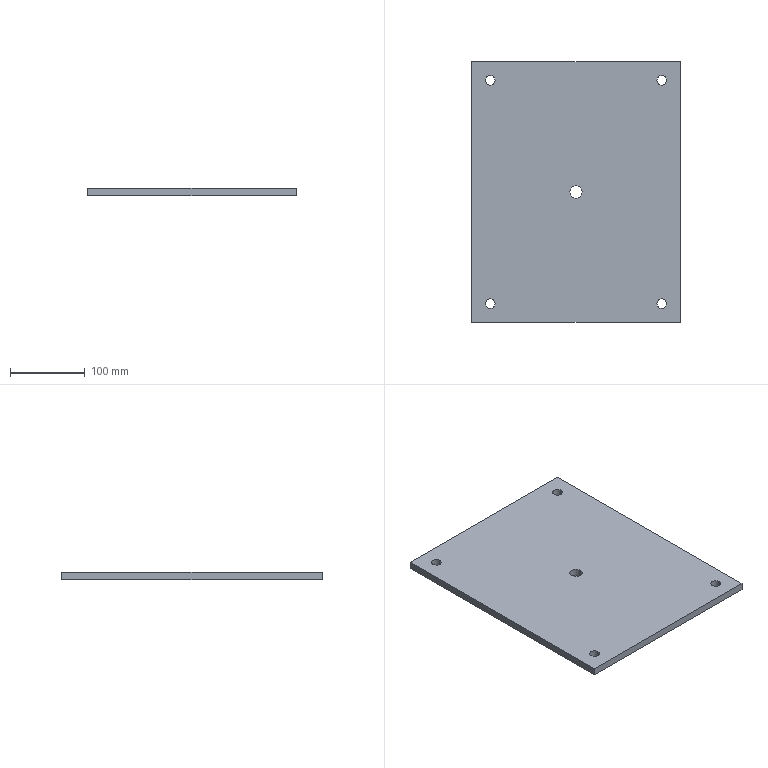Part | STEP file | 44-02-04 Locating Push Plate | 1 solid | 16 faces | box 280 x 350 x 10 mm | volume 972552 mm3 | cylinder 10 | plane 6 | commonest cylinder face diameters 13 x8 16.5 x2
STEP:
#1=CARTESIAN_POINT('',(0.,0.,0.));
#2=DIRECTION('',(0.,0.,1.));
#3=DIRECTION('',(1.,0.,0.));
#4=AXIS2_PLACEMENT_3D('',#1,#2,#3);
#5=CARTESIAN_POINT('',(108.5,150.,10.));
#6=VERTEX_POINT('',#5);
#7=CARTESIAN_POINT('',(108.5,150.,0.));
#8=VERTEX_POINT('',#7);
#9=CARTESIAN_POINT('',(108.5,150.,10.));
#10=DIRECTION('',(0.,0.,-1.));
#11=VECTOR('',#10,1.);
#12=LINE('',#9,#11);
#13=CARTESIAN_POINT('',(115.,150.,10.));
#14=DIRECTION('',(0.,0.,-1.));
#15=DIRECTION('',(-1.,0.,0.));
#16=AXIS2_PLACEMENT_3D('',#13,#14,#15);
#17=CYLINDRICAL_SURFACE('',#16,6.5);
#18=CARTESIAN_POINT('',(6.283,0.));
#19=DIRECTION('',(0.,1.));
#20=VECTOR('',#19,1.);
#21=LINE('',#18,#20);
#22=(GEOMETRIC_REPRESENTATION_CONTEXT(2)PARAMETRIC_REPRESENTATION_CONTEXT()REPRESENTATION_CONTEXT('',''));
#23=DEFINITIONAL_REPRESENTATION('',(#21),#22);
#24=PCURVE('',#17,#23);
#25=CARTESIAN_POINT('',(115.,150.,10.));
#26=DIRECTION('',(0.,0.,-1.));
#27=DIRECTION('',(-1.,0.,0.));
#28=AXIS2_PLACEMENT_3D('',#25,#26,#27);
#29=CYLINDRICAL_SURFACE('',#28,6.5);
#30=CARTESIAN_POINT('',(0.,0.));
#31=DIRECTION('',(0.,1.));
#32=VECTOR('',#31,1.);
#33=LINE('',#30,#32);
#34=(GEOMETRIC_REPRESENTATION_CONTEXT(2)PARAMETRIC_REPRESENTATION_CONTEXT()REPRESENTATION_CONTEXT('',''));
#35=DEFINITIONAL_REPRESENTATION('',(#33),#34);
#36=PCURVE('',#29,#35);
#37=SURFACE_CURVE('',#12,(#24,#36),.PCURVE_S1.);
#38=EDGE_CURVE('',#6,#8,#37,.T.);
#39=ORIENTED_EDGE('',*,*,#38,.T.);
#40=CARTESIAN_POINT('',(121.5,150.,0.));
#41=VERTEX_POINT('',#40);
#42=CARTESIAN_POINT('',(115.,150.,0.));
#43=DIRECTION('',(0.,0.,1.));
#44=DIRECTION('',(1.,0.,0.));
#45=AXIS2_PLACEMENT_3D('',#42,#43,#44);
#46=CIRCLE('',#45,6.5);
#47=CARTESIAN_POINT('',(9.425,10.));
#48=DIRECTION('',(-1.,0.));
#49=VECTOR('',#48,1.);
#50=LINE('',#47,#49);
#51=(GEOMETRIC_REPRESENTATION_CONTEXT(2)PARAMETRIC_REPRESENTATION_CONTEXT()REPRESENTATION_CONTEXT('',''));
#52=DEFINITIONAL_REPRESENTATION('',(#50),#51);
#53=PCURVE('',#17,#52);
#54=CARTESIAN_POINT('',(140.,-175.,0.));
#55=DIRECTION('',(0.,0.,1.));
#56=DIRECTION('',(1.,0.,0.));
#57=AXIS2_PLACEMENT_3D('',#54,#55,#56);
#58=PLANE('',#57);
#59=CARTESIAN_POINT('',(-25.,325.));
#60=DIRECTION('',(1.,0.));
#61=AXIS2_PLACEMENT_2D('',#59,#60);
#62=CIRCLE('',#61,6.5);
#63=(GEOMETRIC_REPRESENTATION_CONTEXT(2)PARAMETRIC_REPRESENTATION_CONTEXT()REPRESENTATION_CONTEXT('',''));
#64=DEFINITIONAL_REPRESENTATION('',(#62),#63);
#65=PCURVE('',#58,#64);
#66=SURFACE_CURVE('',#46,(#53,#65),.PCURVE_S1.);
#67=EDGE_CURVE('',#8,#41,#66,.T.);
#68=ORIENTED_EDGE('',*,*,#67,.T.);
#69=CARTESIAN_POINT('',(121.5,150.,10.));
#70=VERTEX_POINT('',#69);
#71=CARTESIAN_POINT('',(121.5,150.,10.));
#72=DIRECTION('',(0.,0.,-1.));
#73=VECTOR('',#72,1.);
#74=LINE('',#71,#73);
#75=CARTESIAN_POINT('',(3.142,0.));
#76=DIRECTION('',(0.,1.));
#77=VECTOR('',#76,1.);
#78=LINE('',#75,#77);
#79=(GEOMETRIC_REPRESENTATION_CONTEXT(2)PARAMETRIC_REPRESENTATION_CONTEXT()REPRESENTATION_CONTEXT('',''));
#80=DEFINITIONAL_REPRESENTATION('',(#78),#79);
#81=PCURVE('',#17,#80);
#82=CARTESIAN_POINT('',(3.142,0.));
#83=DIRECTION('',(0.,1.));
#84=VECTOR('',#83,1.);
#85=LINE('',#82,#84);
#86=(GEOMETRIC_REPRESENTATION_CONTEXT(2)PARAMETRIC_REPRESENTATION_CONTEXT()REPRESENTATION_CONTEXT('',''));
#87=DEFINITIONAL_REPRESENTATION('',(#85),#86);
#88=PCURVE('',#29,#87);
#89=SURFACE_CURVE('',#74,(#81,#88),.PCURVE_S1.);
#90=EDGE_CURVE('',#70,#41,#89,.T.);
#91=ORIENTED_EDGE('',*,*,#90,.F.);
#92=CARTESIAN_POINT('',(115.,150.,10.));
#93=DIRECTION('',(0.,0.,1.));
#94=DIRECTION('',(1.,0.,0.));
#95=AXIS2_PLACEMENT_3D('',#92,#93,#94);
#96=CIRCLE('',#95,6.5);
#97=CARTESIAN_POINT('',(9.425,0.));
#98=DIRECTION('',(-1.,0.));
#99=VECTOR('',#98,1.);
#100=LINE('',#97,#99);
#101=(GEOMETRIC_REPRESENTATION_CONTEXT(2)PARAMETRIC_REPRESENTATION_CONTEXT()REPRESENTATION_CONTEXT('',''));
#102=DEFINITIONAL_REPRESENTATION('',(#100),#101);
#103=PCURVE('',#17,#102);
#104=CARTESIAN_POINT('',(140.,-175.,10.));
#105=DIRECTION('',(0.,0.,1.));
#106=DIRECTION('',(1.,0.,0.));
#107=AXIS2_PLACEMENT_3D('',#104,#105,#106);
#108=PLANE('',#107);
#109=CARTESIAN_POINT('',(-25.,325.));
#110=DIRECTION('',(1.,0.));
#111=AXIS2_PLACEMENT_2D('',#109,#110);
#112=CIRCLE('',#111,6.5);
#113=(GEOMETRIC_REPRESENTATION_CONTEXT(2)PARAMETRIC_REPRESENTATION_CONTEXT()REPRESENTATION_CONTEXT('',''));
#114=DEFINITIONAL_REPRESENTATION('',(#112),#113);
#115=PCURVE('',#108,#114);
#116=SURFACE_CURVE('',#96,(#103,#115),.PCURVE_S1.);
#117=EDGE_CURVE('',#6,#70,#116,.T.);
#118=ORIENTED_EDGE('',*,*,#117,.F.);
#119=EDGE_LOOP('',(#39,#68,#91,#118));
#120=FACE_BOUND('',#119,.F.);
#121=ADVANCED_FACE('',(#120),#17,.F.);
#122=CARTESIAN_POINT('',(-121.5,150.,10.));
#123=VERTEX_POINT('',#122);
#124=CARTESIAN_POINT('',(-121.5,150.,0.));
#125=VERTEX_POINT('',#124);
#126=CARTESIAN_POINT('',(-121.5,150.,10.));
#127=DIRECTION('',(0.,0.,-1.));
#128=VECTOR('',#127,1.);
#129=LINE('',#126,#128);
#130=CARTESIAN_POINT('',(-115.,150.,10.));
#131=DIRECTION('',(0.,0.,-1.));
#132=DIRECTION('',(-1.,0.,0.));
#133=AXIS2_PLACEMENT_3D('',#130,#131,#132);
#134=CYLINDRICAL_SURFACE('',#133,6.5);
#135=CARTESIAN_POINT('',(6.283,0.));
#136=DIRECTION('',(0.,1.));
#137=VECTOR('',#136,1.);
#138=LINE('',#135,#137);
#139=(GEOMETRIC_REPRESENTATION_CONTEXT(2)PARAMETRIC_REPRESENTATION_CONTEXT()REPRESENTATION_CONTEXT('',''));
#140=DEFINITIONAL_REPRESENTATION('',(#138),#139);
#141=PCURVE('',#134,#140);
#142=CARTESIAN_POINT('',(-115.,150.,10.));
#143=DIRECTION('',(0.,0.,-1.));
#144=DIRECTION('',(-1.,0.,0.));
#145=AXIS2_PLACEMENT_3D('',#142,#143,#144);
#146=CYLINDRICAL_SURFACE('',#145,6.5);
#147=CARTESIAN_POINT('',(0.,0.));
#148=DIRECTION('',(0.,1.));
#149=VECTOR('',#148,1.);
#150=LINE('',#147,#149);
#151=(GEOMETRIC_REPRESENTATION_CONTEXT(2)PARAMETRIC_REPRESENTATION_CONTEXT()REPRESENTATION_CONTEXT('',''));
#152=DEFINITIONAL_REPRESENTATION('',(#150),#151);
#153=PCURVE('',#146,#152);
#154=SURFACE_CURVE('',#129,(#141,#153),.PCURVE_S1.);
#155=EDGE_CURVE('',#123,#125,#154,.T.);
#156=ORIENTED_EDGE('',*,*,#155,.T.);
#157=CARTESIAN_POINT('',(-108.5,150.,0.));
#158=VERTEX_POINT('',#157);
#159=CARTESIAN_POINT('',(-115.,150.,0.));
#160=DIRECTION('',(0.,0.,1.));
#161=DIRECTION('',(1.,0.,0.));
#162=AXIS2_PLACEMENT_3D('',#159,#160,#161);
#163=CIRCLE('',#162,6.5);
#164=CARTESIAN_POINT('',(9.425,10.));
#165=DIRECTION('',(-1.,0.));
#166=VECTOR('',#165,1.);
#167=LINE('',#164,#166);
#168=(GEOMETRIC_REPRESENTATION_CONTEXT(2)PARAMETRIC_REPRESENTATION_CONTEXT()REPRESENTATION_CONTEXT('',''));
#169=DEFINITIONAL_REPRESENTATION('',(#167),#168);
#170=PCURVE('',#134,#169);
#171=CARTESIAN_POINT('',(-255.,325.));
#172=DIRECTION('',(1.,0.));
#173=AXIS2_PLACEMENT_2D('',#171,#172);
#174=CIRCLE('',#173,6.5);
#175=(GEOMETRIC_REPRESENTATION_CONTEXT(2)PARAMETRIC_REPRESENTATION_CONTEXT()REPRESENTATION_CONTEXT('',''));
#176=DEFINITIONAL_REPRESENTATION('',(#174),#175);
#177=PCURVE('',#58,#176);
#178=SURFACE_CURVE('',#163,(#170,#177),.PCURVE_S1.);
#179=EDGE_CURVE('',#125,#158,#178,.T.);
#180=ORIENTED_EDGE('',*,*,#179,.T.);
#181=CARTESIAN_POINT('',(-108.5,150.,10.));
#182=VERTEX_POINT('',#181);
#183=CARTESIAN_POINT('',(-108.5,150.,10.));
#184=DIRECTION('',(0.,0.,-1.));
#185=VECTOR('',#184,1.);
#186=LINE('',#183,#185);
#187=CARTESIAN_POINT('',(3.142,0.));
#188=DIRECTION('',(0.,1.));
#189=VECTOR('',#188,1.);
#190=LINE('',#187,#189);
#191=(GEOMETRIC_REPRESENTATION_CONTEXT(2)PARAMETRIC_REPRESENTATION_CONTEXT()REPRESENTATION_CONTEXT('',''));
#192=DEFINITIONAL_REPRESENTATION('',(#190),#191);
#193=PCURVE('',#134,#192);
#194=CARTESIAN_POINT('',(3.142,0.));
#195=DIRECTION('',(0.,1.));
#196=VECTOR('',#195,1.);
#197=LINE('',#194,#196);
#198=(GEOMETRIC_REPRESENTATION_CONTEXT(2)PARAMETRIC_REPRESENTATION_CONTEXT()REPRESENTATION_CONTEXT('',''));
#199=DEFINITIONAL_REPRESENTATION('',(#197),#198);
#200=PCURVE('',#146,#199);
#201=SURFACE_CURVE('',#186,(#193,#200),.PCURVE_S1.);
#202=EDGE_CURVE('',#182,#158,#201,.T.);
#203=ORIENTED_EDGE('',*,*,#202,.F.);
#204=CARTESIAN_POINT('',(-115.,150.,10.));
#205=DIRECTION('',(0.,0.,1.));
#206=DIRECTION('',(1.,0.,0.));
#207=AXIS2_PLACEMENT_3D('',#204,#205,#206);
#208=CIRCLE('',#207,6.5);
#209=CARTESIAN_POINT('',(9.425,0.));
#210=DIRECTION('',(-1.,0.));
#211=VECTOR('',#210,1.);
#212=LINE('',#209,#211);
#213=(GEOMETRIC_REPRESENTATION_CONTEXT(2)PARAMETRIC_REPRESENTATION_CONTEXT()REPRESENTATION_CONTEXT('',''));
#214=DEFINITIONAL_REPRESENTATION('',(#212),#213);
#215=PCURVE('',#134,#214);
#216=CARTESIAN_POINT('',(-255.,325.));
#217=DIRECTION('',(1.,0.));
#218=AXIS2_PLACEMENT_2D('',#216,#217);
#219=CIRCLE('',#218,6.5);
#220=(GEOMETRIC_REPRESENTATION_CONTEXT(2)PARAMETRIC_REPRESENTATION_CONTEXT()REPRESENTATION_CONTEXT('',''));
#221=DEFINITIONAL_REPRESENTATION('',(#219),#220);
#222=PCURVE('',#108,#221);
#223=SURFACE_CURVE('',#208,(#215,#222),.PCURVE_S1.);
#224=EDGE_CURVE('',#123,#182,#223,.T.);
#225=ORIENTED_EDGE('',*,*,#224,.F.);
#226=EDGE_LOOP('',(#156,#180,#203,#225));
#227=FACE_BOUND('',#226,.F.);
#228=ADVANCED_FACE('',(#227),#134,.F.);
#229=CARTESIAN_POINT('',(108.5,-150.,10.));
#230=VERTEX_POINT('',#229);
#231=CARTESIAN_POINT('',(108.5,-150.,0.));
#232=VERTEX_POINT('',#231);
#233=CARTESIAN_POINT('',(108.5,-150.,10.));
#234=DIRECTION('',(0.,0.,-1.));
#235=VECTOR('',#234,1.);
#236=LINE('',#233,#235);
#237=CARTESIAN_POINT('',(115.,-150.,10.));
#238=DIRECTION('',(0.,0.,-1.));
#239=DIRECTION('',(-1.,0.,0.));
#240=AXIS2_PLACEMENT_3D('',#237,#238,#239);
#241=CYLINDRICAL_SURFACE('',#240,6.5);
#242=CARTESIAN_POINT('',(6.283,0.));
#243=DIRECTION('',(0.,1.));
#244=VECTOR('',#243,1.);
#245=LINE('',#242,#244);
#246=(GEOMETRIC_REPRESENTATION_CONTEXT(2)PARAMETRIC_REPRESENTATION_CONTEXT()REPRESENTATION_CONTEXT('',''));
#247=DEFINITIONAL_REPRESENTATION('',(#245),#246);
#248=PCURVE('',#241,#247);
#249=CARTESIAN_POINT('',(115.,-150.,10.));
#250=DIRECTION('',(0.,0.,-1.));
#251=DIRECTION('',(-1.,0.,0.));
#252=AXIS2_PLACEMENT_3D('',#249,#250,#251);
#253=CYLINDRICAL_SURFACE('',#252,6.5);
#254=CARTESIAN_POINT('',(0.,0.));
#255=DIRECTION('',(0.,1.));
#256=VECTOR('',#255,1.);
#257=LINE('',#254,#256);
#258=(GEOMETRIC_REPRESENTATION_CONTEXT(2)PARAMETRIC_REPRESENTATION_CONTEXT()REPRESENTATION_CONTEXT('',''));
#259=DEFINITIONAL_REPRESENTATION('',(#257),#258);
#260=PCURVE('',#253,#259);
#261=SURFACE_CURVE('',#236,(#248,#260),.PCURVE_S1.);
#262=EDGE_CURVE('',#230,#232,#261,.T.);
#263=ORIENTED_EDGE('',*,*,#262,.T.);
#264=CARTESIAN_POINT('',(121.5,-150.,0.));
#265=VERTEX_POINT('',#264);
#266=CARTESIAN_POINT('',(115.,-150.,0.));
#267=DIRECTION('',(0.,0.,1.));
#268=DIRECTION('',(1.,0.,0.));
#269=AXIS2_PLACEMENT_3D('',#266,#267,#268);
#270=CIRCLE('',#269,6.5);
#271=CARTESIAN_POINT('',(9.425,10.));
#272=DIRECTION('',(-1.,0.));
#273=VECTOR('',#272,1.);
#274=LINE('',#271,#273);
#275=(GEOMETRIC_REPRESENTATION_CONTEXT(2)PARAMETRIC_REPRESENTATION_CONTEXT()REPRESENTATION_CONTEXT('',''));
#276=DEFINITIONAL_REPRESENTATION('',(#274),#275);
#277=PCURVE('',#241,#276);
#278=CARTESIAN_POINT('',(-25.,25.));
#279=DIRECTION('',(1.,0.));
#280=AXIS2_PLACEMENT_2D('',#278,#279);
#281=CIRCLE('',#280,6.5);
#282=(GEOMETRIC_REPRESENTATION_CONTEXT(2)PARAMETRIC_REPRESENTATION_CONTEXT()REPRESENTATION_CONTEXT('',''));
#283=DEFINITIONAL_REPRESENTATION('',(#281),#282);
#284=PCURVE('',#58,#283);
#285=SURFACE_CURVE('',#270,(#277,#284),.PCURVE_S1.);
#286=EDGE_CURVE('',#232,#265,#285,.T.);
#287=ORIENTED_EDGE('',*,*,#286,.T.);
#288=CARTESIAN_POINT('',(121.5,-150.,10.));
#289=VERTEX_POINT('',#288);
#290=CARTESIAN_POINT('',(121.5,-150.,10.));
#291=DIRECTION('',(0.,0.,-1.));
#292=VECTOR('',#291,1.);
#293=LINE('',#290,#292);
#294=CARTESIAN_POINT('',(3.142,0.));
#295=DIRECTION('',(0.,1.));
#296=VECTOR('',#295,1.);
#297=LINE('',#294,#296);
#298=(GEOMETRIC_REPRESENTATION_CONTEXT(2)PARAMETRIC_REPRESENTATION_CONTEXT()REPRESENTATION_CONTEXT('',''));
#299=DEFINITIONAL_REPRESENTATION('',(#297),#298);
#300=PCURVE('',#241,#299);
#301=CARTESIAN_POINT('',(3.142,0.));
#302=DIRECTION('',(0.,1.));
#303=VECTOR('',#302,1.);
#304=LINE('',#301,#303);
#305=(GEOMETRIC_REPRESENTATION_CONTEXT(2)PARAMETRIC_REPRESENTATION_CONTEXT()REPRESENTATION_CONTEXT('',''));
#306=DEFINITIONAL_REPRESENTATION('',(#304),#305);
#307=PCURVE('',#253,#306);
#308=SURFACE_CURVE('',#293,(#300,#307),.PCURVE_S1.);
#309=EDGE_CURVE('',#289,#265,#308,.T.);
#310=ORIENTED_EDGE('',*,*,#309,.F.);
#311=CARTESIAN_POINT('',(115.,-150.,10.));
#312=DIRECTION('',(0.,0.,1.));
#313=DIRECTION('',(1.,0.,0.));
#314=AXIS2_PLACEMENT_3D('',#311,#312,#313);
#315=CIRCLE('',#314,6.5);
#316=CARTESIAN_POINT('',(9.425,0.));
#317=DIRECTION('',(-1.,0.));
#318=VECTOR('',#317,1.);
#319=LINE('',#316,#318);
#320=(GEOMETRIC_REPRESENTATION_CONTEXT(2)PARAMETRIC_REPRESENTATION_CONTEXT()REPRESENTATION_CONTEXT('',''));
#321=DEFINITIONAL_REPRESENTATION('',(#319),#320);
#322=PCURVE('',#241,#321);
#323=CARTESIAN_POINT('',(-25.,25.));
#324=DIRECTION('',(1.,0.));
#325=AXIS2_PLACEMENT_2D('',#323,#324);
#326=CIRCLE('',#325,6.5);
#327=(GEOMETRIC_REPRESENTATION_CONTEXT(2)PARAMETRIC_REPRESENTATION_CONTEXT()REPRESENTATION_CONTEXT('',''));
#328=DEFINITIONAL_REPRESENTATION('',(#326),#327);
#329=PCURVE('',#108,#328);
#330=SURFACE_CURVE('',#315,(#322,#329),.PCURVE_S1.);
#331=EDGE_CURVE('',#230,#289,#330,.T.);
#332=ORIENTED_EDGE('',*,*,#331,.F.);
#333=EDGE_LOOP('',(#263,#287,#310,#332));
#334=FACE_BOUND('',#333,.F.);
#335=ADVANCED_FACE('',(#334),#241,.F.);
#336=CARTESIAN_POINT('',(-121.5,-150.,10.));
#337=VERTEX_POINT('',#336);
#338=CARTESIAN_POINT('',(-121.5,-150.,0.));
#339=VERTEX_POINT('',#338);
#340=CARTESIAN_POINT('',(-121.5,-150.,10.));
#341=DIRECTION('',(0.,0.,-1.));
#342=VECTOR('',#341,1.);
#343=LINE('',#340,#342);
#344=CARTESIAN_POINT('',(-115.,-150.,10.));
#345=DIRECTION('',(0.,0.,-1.));
#346=DIRECTION('',(-1.,0.,0.));
#347=AXIS2_PLACEMENT_3D('',#344,#345,#346);
#348=CYLINDRICAL_SURFACE('',#347,6.5);
#349=CARTESIAN_POINT('',(6.283,0.));
#350=DIRECTION('',(0.,1.));
#351=VECTOR('',#350,1.);
#352=LINE('',#349,#351);
#353=(GEOMETRIC_REPRESENTATION_CONTEXT(2)PARAMETRIC_REPRESENTATION_CONTEXT()REPRESENTATION_CONTEXT('',''));
#354=DEFINITIONAL_REPRESENTATION('',(#352),#353);
#355=PCURVE('',#348,#354);
#356=CARTESIAN_POINT('',(-115.,-150.,10.));
#357=DIRECTION('',(0.,0.,-1.));
#358=DIRECTION('',(-1.,0.,0.));
#359=AXIS2_PLACEMENT_3D('',#356,#357,#358);
#360=CYLINDRICAL_SURFACE('',#359,6.5);
#361=CARTESIAN_POINT('',(0.,0.));
#362=DIRECTION('',(0.,1.));
#363=VECTOR('',#362,1.);
#364=LINE('',#361,#363);
#365=(GEOMETRIC_REPRESENTATION_CONTEXT(2)PARAMETRIC_REPRESENTATION_CONTEXT()REPRESENTATION_CONTEXT('',''));
#366=DEFINITIONAL_REPRESENTATION('',(#364),#365);
#367=PCURVE('',#360,#366);
#368=SURFACE_CURVE('',#343,(#355,#367),.PCURVE_S1.);
#369=EDGE_CURVE('',#337,#339,#368,.T.);
#370=ORIENTED_EDGE('',*,*,#369,.T.);
#371=CARTESIAN_POINT('',(-108.5,-150.,0.));
#372=VERTEX_POINT('',#371);
#373=CARTESIAN_POINT('',(-115.,-150.,0.));
#374=DIRECTION('',(0.,0.,1.));
#375=DIRECTION('',(1.,0.,0.));
#376=AXIS2_PLACEMENT_3D('',#373,#374,#375);
#377=CIRCLE('',#376,6.5);
#378=CARTESIAN_POINT('',(9.425,10.));
#379=DIRECTION('',(-1.,0.));
#380=VECTOR('',#379,1.);
#381=LINE('',#378,#380);
#382=(GEOMETRIC_REPRESENTATION_CONTEXT(2)PARAMETRIC_REPRESENTATION_CONTEXT()REPRESENTATION_CONTEXT('',''));
#383=DEFINITIONAL_REPRESENTATION('',(#381),#382);
#384=PCURVE('',#348,#383);
#385=CARTESIAN_POINT('',(-255.,25.));
#386=DIRECTION('',(1.,0.));
#387=AXIS2_PLACEMENT_2D('',#385,#386);
#388=CIRCLE('',#387,6.5);
#389=(GEOMETRIC_REPRESENTATION_CONTEXT(2)PARAMETRIC_REPRESENTATION_CONTEXT()REPRESENTATION_CONTEXT('',''));
#390=DEFINITIONAL_REPRESENTATION('',(#388),#389);
#391=PCURVE('',#58,#390);
#392=SURFACE_CURVE('',#377,(#384,#391),.PCURVE_S1.);
#393=EDGE_CURVE('',#339,#372,#392,.T.);
#394=ORIENTED_EDGE('',*,*,#393,.T.);
#395=CARTESIAN_POINT('',(-108.5,-150.,10.));
#396=VERTEX_POINT('',#395);
#397=CARTESIAN_POINT('',(-108.5,-150.,10.));
#398=DIRECTION('',(0.,0.,-1.));
#399=VECTOR('',#398,1.);
#400=LINE('',#397,#399);
#401=CARTESIAN_POINT('',(3.142,0.));
#402=DIRECTION('',(0.,1.));
#403=VECTOR('',#402,1.);
#404=LINE('',#401,#403);
#405=(GEOMETRIC_REPRESENTATION_CONTEXT(2)PARAMETRIC_REPRESENTATION_CONTEXT()REPRESENTATION_CONTEXT('',''));
#406=DEFINITIONAL_REPRESENTATION('',(#404),#405);
#407=PCURVE('',#348,#406);
#408=CARTESIAN_POINT('',(3.142,0.));
#409=DIRECTION('',(0.,1.));
#410=VECTOR('',#409,1.);
#411=LINE('',#408,#410);
#412=(GEOMETRIC_REPRESENTATION_CONTEXT(2)PARAMETRIC_REPRESENTATION_CONTEXT()REPRESENTATION_CONTEXT('',''));
#413=DEFINITIONAL_REPRESENTATION('',(#411),#412);
#414=PCURVE('',#360,#413);
#415=SURFACE_CURVE('',#400,(#407,#414),.PCURVE_S1.);
#416=EDGE_CURVE('',#396,#372,#415,.T.);
#417=ORIENTED_EDGE('',*,*,#416,.F.);
#418=CARTESIAN_POINT('',(-115.,-150.,10.));
#419=DIRECTION('',(0.,0.,1.));
#420=DIRECTION('',(1.,0.,0.));
#421=AXIS2_PLACEMENT_3D('',#418,#419,#420);
#422=CIRCLE('',#421,6.5);
#423=CARTESIAN_POINT('',(9.425,0.));
#424=DIRECTION('',(-1.,0.));
#425=VECTOR('',#424,1.);
#426=LINE('',#423,#425);
#427=(GEOMETRIC_REPRESENTATION_CONTEXT(2)PARAMETRIC_REPRESENTATION_CONTEXT()REPRESENTATION_CONTEXT('',''));
#428=DEFINITIONAL_REPRESENTATION('',(#426),#427);
#429=PCURVE('',#348,#428);
#430=CARTESIAN_POINT('',(-255.,25.));
#431=DIRECTION('',(1.,0.));
#432=AXIS2_PLACEMENT_2D('',#430,#431);
#433=CIRCLE('',#432,6.5);
#434=(GEOMETRIC_REPRESENTATION_CONTEXT(2)PARAMETRIC_REPRESENTATION_CONTEXT()REPRESENTATION_CONTEXT('',''));
#435=DEFINITIONAL_REPRESENTATION('',(#433),#434);
#436=PCURVE('',#108,#435);
#437=SURFACE_CURVE('',#422,(#429,#436),.PCURVE_S1.);
#438=EDGE_CURVE('',#337,#396,#437,.T.);
#439=ORIENTED_EDGE('',*,*,#438,.F.);
#440=EDGE_LOOP('',(#370,#394,#417,#439));
#441=FACE_BOUND('',#440,.F.);
#442=ADVANCED_FACE('',(#441),#348,.F.);
#443=CARTESIAN_POINT('',(8.25,0.,0.));
#444=VERTEX_POINT('',#443);
#445=CARTESIAN_POINT('',(8.25,0.,10.));
#446=VERTEX_POINT('',#445);
#447=CARTESIAN_POINT('',(8.25,0.,10.));
#448=DIRECTION('',(0.,0.,1.));
#449=VECTOR('',#448,1.);
#450=LINE('',#447,#449);
#451=CARTESIAN_POINT('',(0.,0.,10.));
#452=DIRECTION('',(0.,0.,1.));
#453=DIRECTION('',(1.,0.,0.));
#454=AXIS2_PLACEMENT_3D('',#451,#452,#453);
#455=CYLINDRICAL_SURFACE('',#454,8.25);
#456=CARTESIAN_POINT('',(6.283,0.));
#457=DIRECTION('',(0.,1.));
#458=VECTOR('',#457,1.);
#459=LINE('',#456,#458);
#460=(GEOMETRIC_REPRESENTATION_CONTEXT(2)PARAMETRIC_REPRESENTATION_CONTEXT()REPRESENTATION_CONTEXT('',''));
#461=DEFINITIONAL_REPRESENTATION('',(#459),#460);
#462=PCURVE('',#455,#461);
#463=CARTESIAN_POINT('',(0.,0.,10.));
#464=DIRECTION('',(0.,0.,1.));
#465=DIRECTION('',(1.,0.,0.));
#466=AXIS2_PLACEMENT_3D('',#463,#464,#465);
#467=CYLINDRICAL_SURFACE('',#466,8.25);
#468=CARTESIAN_POINT('',(0.,0.));
#469=DIRECTION('',(0.,1.));
#470=VECTOR('',#469,1.);
#471=LINE('',#468,#470);
#472=(GEOMETRIC_REPRESENTATION_CONTEXT(2)PARAMETRIC_REPRESENTATION_CONTEXT()REPRESENTATION_CONTEXT('',''));
#473=DEFINITIONAL_REPRESENTATION('',(#471),#472);
#474=PCURVE('',#467,#473);
#475=SURFACE_CURVE('',#450,(#462,#474),.PCURVE_S1.);
#476=EDGE_CURVE('',#444,#446,#475,.T.);
#477=ORIENTED_EDGE('',*,*,#476,.T.);
#478=CARTESIAN_POINT('',(-8.25,0.,10.));
#479=VERTEX_POINT('',#478);
#480=CARTESIAN_POINT('',(0.,0.,10.));
#481=DIRECTION('',(0.,0.,1.));
#482=DIRECTION('',(1.,0.,0.));
#483=AXIS2_PLACEMENT_3D('',#480,#481,#482);
#484=CIRCLE('',#483,8.25);
#485=CARTESIAN_POINT('',(0.,0.));
#486=DIRECTION('',(1.,0.));
#487=VECTOR('',#486,1.);
#488=LINE('',#485,#487);
#489=(GEOMETRIC_REPRESENTATION_CONTEXT(2)PARAMETRIC_REPRESENTATION_CONTEXT()REPRESENTATION_CONTEXT('',''));
#490=DEFINITIONAL_REPRESENTATION('',(#488),#489);
#491=PCURVE('',#455,#490);
#492=CARTESIAN_POINT('',(-140.,175.));
#493=DIRECTION('',(1.,0.));
#494=AXIS2_PLACEMENT_2D('',#492,#493);
#495=CIRCLE('',#494,8.25);
#496=(GEOMETRIC_REPRESENTATION_CONTEXT(2)PARAMETRIC_REPRESENTATION_CONTEXT()REPRESENTATION_CONTEXT('',''));
#497=DEFINITIONAL_REPRESENTATION('',(#495),#496);
#498=PCURVE('',#108,#497);
#499=SURFACE_CURVE('',#484,(#491,#498),.PCURVE_S1.);
#500=EDGE_CURVE('',#479,#446,#499,.T.);
#501=ORIENTED_EDGE('',*,*,#500,.F.);
#502=CARTESIAN_POINT('',(-8.25,0.,0.));
#503=VERTEX_POINT('',#502);
#504=CARTESIAN_POINT('',(-8.25,0.,10.));
#505=DIRECTION('',(0.,0.,1.));
#506=VECTOR('',#505,1.);
#507=LINE('',#504,#506);
#508=CARTESIAN_POINT('',(3.142,0.));
#509=DIRECTION('',(0.,1.));
#510=VECTOR('',#509,1.);
#511=LINE('',#508,#510);
#512=(GEOMETRIC_REPRESENTATION_CONTEXT(2)PARAMETRIC_REPRESENTATION_CONTEXT()REPRESENTATION_CONTEXT('',''));
#513=DEFINITIONAL_REPRESENTATION('',(#511),#512);
#514=PCURVE('',#455,#513);
#515=CARTESIAN_POINT('',(3.142,0.));
#516=DIRECTION('',(0.,1.));
#517=VECTOR('',#516,1.);
#518=LINE('',#515,#517);
#519=(GEOMETRIC_REPRESENTATION_CONTEXT(2)PARAMETRIC_REPRESENTATION_CONTEXT()REPRESENTATION_CONTEXT('',''));
#520=DEFINITIONAL_REPRESENTATION('',(#518),#519);
#521=PCURVE('',#467,#520);
#522=SURFACE_CURVE('',#507,(#514,#521),.PCURVE_S1.);
#523=EDGE_CURVE('',#503,#479,#522,.T.);
#524=ORIENTED_EDGE('',*,*,#523,.F.);
#525=CARTESIAN_POINT('',(0.,0.,0.));
#526=DIRECTION('',(0.,0.,1.));
#527=DIRECTION('',(1.,0.,0.));
#528=AXIS2_PLACEMENT_3D('',#525,#526,#527);
#529=CIRCLE('',#528,8.25);
#530=CARTESIAN_POINT('',(0.,-10.));
#531=DIRECTION('',(1.,0.));
#532=VECTOR('',#531,1.);
#533=LINE('',#530,#532);
#534=(GEOMETRIC_REPRESENTATION_CONTEXT(2)PARAMETRIC_REPRESENTATION_CONTEXT()REPRESENTATION_CONTEXT('',''));
#535=DEFINITIONAL_REPRESENTATION('',(#533),#534);
#536=PCURVE('',#455,#535);
#537=CARTESIAN_POINT('',(-140.,175.));
#538=DIRECTION('',(1.,0.));
#539=AXIS2_PLACEMENT_2D('',#537,#538);
#540=CIRCLE('',#539,8.25);
#541=(GEOMETRIC_REPRESENTATION_CONTEXT(2)PARAMETRIC_REPRESENTATION_CONTEXT()REPRESENTATION_CONTEXT('',''));
#542=DEFINITIONAL_REPRESENTATION('',(#540),#541);
#543=PCURVE('',#58,#542);
#544=SURFACE_CURVE('',#529,(#536,#543),.PCURVE_S1.);
#545=EDGE_CURVE('',#503,#444,#544,.T.);
#546=ORIENTED_EDGE('',*,*,#545,.T.);
#547=EDGE_LOOP('',(#477,#501,#524,#546));
#548=FACE_BOUND('',#547,.F.);
#549=ADVANCED_FACE('',(#548),#455,.F.);
#550=ORIENTED_EDGE('',*,*,#224,.F.);
#551=CARTESIAN_POINT('',(-115.,150.,10.));
#552=DIRECTION('',(0.,0.,1.));
#553=DIRECTION('',(1.,0.,0.));
#554=AXIS2_PLACEMENT_3D('',#551,#552,#553);
#555=CIRCLE('',#554,6.5);
#556=CARTESIAN_POINT('',(-255.,325.));
#557=DIRECTION('',(1.,0.));
#558=AXIS2_PLACEMENT_2D('',#556,#557);
#559=CIRCLE('',#558,6.5);
#560=(GEOMETRIC_REPRESENTATION_CONTEXT(2)PARAMETRIC_REPRESENTATION_CONTEXT()REPRESENTATION_CONTEXT('',''));
#561=DEFINITIONAL_REPRESENTATION('',(#559),#560);
#562=PCURVE('',#108,#561);
#563=CARTESIAN_POINT('',(3.142,0.));
#564=DIRECTION('',(-1.,0.));
#565=VECTOR('',#564,1.);
#566=LINE('',#563,#565);
#567=(GEOMETRIC_REPRESENTATION_CONTEXT(2)PARAMETRIC_REPRESENTATION_CONTEXT()REPRESENTATION_CONTEXT('',''));
#568=DEFINITIONAL_REPRESENTATION('',(#566),#567);
#569=PCURVE('',#146,#568);
#570=SURFACE_CURVE('',#555,(#562,#569),.PCURVE_S1.);
#571=EDGE_CURVE('',#182,#123,#570,.T.);
#572=ORIENTED_EDGE('',*,*,#571,.F.);
#573=EDGE_LOOP('',(#550,#572));
#574=FACE_BOUND('',#573,.T.);
#575=ORIENTED_EDGE('',*,*,#438,.F.);
#576=CARTESIAN_POINT('',(-115.,-150.,10.));
#577=DIRECTION('',(0.,0.,1.));
#578=DIRECTION('',(1.,0.,0.));
#579=AXIS2_PLACEMENT_3D('',#576,#577,#578);
#580=CIRCLE('',#579,6.5);
#581=CARTESIAN_POINT('',(-255.,25.));
#582=DIRECTION('',(1.,0.));
#583=AXIS2_PLACEMENT_2D('',#581,#582);
#584=CIRCLE('',#583,6.5);
#585=(GEOMETRIC_REPRESENTATION_CONTEXT(2)PARAMETRIC_REPRESENTATION_CONTEXT()REPRESENTATION_CONTEXT('',''));
#586=DEFINITIONAL_REPRESENTATION('',(#584),#585);
#587=PCURVE('',#108,#586);
#588=CARTESIAN_POINT('',(3.142,0.));
#589=DIRECTION('',(-1.,0.));
#590=VECTOR('',#589,1.);
#591=LINE('',#588,#590);
#592=(GEOMETRIC_REPRESENTATION_CONTEXT(2)PARAMETRIC_REPRESENTATION_CONTEXT()REPRESENTATION_CONTEXT('',''));
#593=DEFINITIONAL_REPRESENTATION('',(#591),#592);
#594=PCURVE('',#360,#593);
#595=SURFACE_CURVE('',#580,(#587,#594),.PCURVE_S1.);
#596=EDGE_CURVE('',#396,#337,#595,.T.);
#597=ORIENTED_EDGE('',*,*,#596,.F.);
#598=EDGE_LOOP('',(#575,#597));
#599=FACE_BOUND('',#598,.T.);
#600=CARTESIAN_POINT('',(0.,0.,10.));
#601=DIRECTION('',(0.,0.,1.));
#602=DIRECTION('',(1.,0.,0.));
#603=AXIS2_PLACEMENT_3D('',#600,#601,#602);
#604=CIRCLE('',#603,8.25);
#605=CARTESIAN_POINT('',(-140.,175.));
#606=DIRECTION('',(1.,0.));
#607=AXIS2_PLACEMENT_2D('',#605,#606);
#608=CIRCLE('',#607,8.25);
#609=(GEOMETRIC_REPRESENTATION_CONTEXT(2)PARAMETRIC_REPRESENTATION_CONTEXT()REPRESENTATION_CONTEXT('',''));
#610=DEFINITIONAL_REPRESENTATION('',(#608),#609);
#611=PCURVE('',#108,#610);
#612=CARTESIAN_POINT('',(0.,0.));
#613=DIRECTION('',(1.,0.));
#614=VECTOR('',#613,1.);
#615=LINE('',#612,#614);
#616=(GEOMETRIC_REPRESENTATION_CONTEXT(2)PARAMETRIC_REPRESENTATION_CONTEXT()REPRESENTATION_CONTEXT('',''));
#617=DEFINITIONAL_REPRESENTATION('',(#615),#616);
#618=PCURVE('',#467,#617);
#619=SURFACE_CURVE('',#604,(#611,#618),.PCURVE_S1.);
#620=EDGE_CURVE('',#446,#479,#619,.T.);
#621=ORIENTED_EDGE('',*,*,#620,.F.);
#622=ORIENTED_EDGE('',*,*,#500,.F.);
#623=EDGE_LOOP('',(#621,#622));
#624=FACE_BOUND('',#623,.T.);
#625=CARTESIAN_POINT('',(140.,-175.,10.));
#626=VERTEX_POINT('',#625);
#627=CARTESIAN_POINT('',(140.,175.,10.));
#628=VERTEX_POINT('',#627);
#629=CARTESIAN_POINT('',(140.,175.,10.));
#630=DIRECTION('',(0.,1.,0.));
#631=VECTOR('',#630,1.);
#632=LINE('',#629,#631);
#633=CARTESIAN_POINT('',(0.,350.));
#634=DIRECTION('',(0.,1.));
#635=VECTOR('',#634,1.);
#636=LINE('',#633,#635);
#637=(GEOMETRIC_REPRESENTATION_CONTEXT(2)PARAMETRIC_REPRESENTATION_CONTEXT()REPRESENTATION_CONTEXT('',''));
#638=DEFINITIONAL_REPRESENTATION('',(#636),#637);
#639=PCURVE('',#108,#638);
#640=CARTESIAN_POINT('',(140.,175.,10.));
#641=DIRECTION('',(-1.,0.,0.));
#642=DIRECTION('',(0.,-1.,0.));
#643=AXIS2_PLACEMENT_3D('',#640,#641,#642);
#644=PLANE('',#643);
#645=CARTESIAN_POINT('',(0.,0.));
#646=DIRECTION('',(-1.,0.));
#647=VECTOR('',#646,1.);
#648=LINE('',#645,#647);
#649=(GEOMETRIC_REPRESENTATION_CONTEXT(2)PARAMETRIC_REPRESENTATION_CONTEXT()REPRESENTATION_CONTEXT('',''));
#650=DEFINITIONAL_REPRESENTATION('',(#648),#649);
#651=PCURVE('',#644,#650);
#652=SURFACE_CURVE('',#632,(#639,#651),.PCURVE_S1.);
#653=EDGE_CURVE('',#626,#628,#652,.T.);
#654=ORIENTED_EDGE('',*,*,#653,.T.);
#655=CARTESIAN_POINT('',(-140.,175.,10.));
#656=VERTEX_POINT('',#655);
#657=CARTESIAN_POINT('',(-140.,175.,10.));
#658=DIRECTION('',(-1.,0.,0.));
#659=VECTOR('',#658,1.);
#660=LINE('',#657,#659);
#661=CARTESIAN_POINT('',(-280.,350.));
#662=DIRECTION('',(-1.,0.));
#663=VECTOR('',#662,1.);
#664=LINE('',#661,#663);
#665=(GEOMETRIC_REPRESENTATION_CONTEXT(2)PARAMETRIC_REPRESENTATION_CONTEXT()REPRESENTATION_CONTEXT('',''));
#666=DEFINITIONAL_REPRESENTATION('',(#664),#665);
#667=PCURVE('',#108,#666);
#668=CARTESIAN_POINT('',(-140.,175.,10.));
#669=DIRECTION('',(0.,-1.,0.));
#670=DIRECTION('',(0.,0.,-1.));
#671=AXIS2_PLACEMENT_3D('',#668,#669,#670);
#672=PLANE('',#671);
#673=CARTESIAN_POINT('',(0.,0.));
#674=DIRECTION('',(0.,-1.));
#675=VECTOR('',#674,1.);
#676=LINE('',#673,#675);
#677=(GEOMETRIC_REPRESENTATION_CONTEXT(2)PARAMETRIC_REPRESENTATION_CONTEXT()REPRESENTATION_CONTEXT('',''));
#678=DEFINITIONAL_REPRESENTATION('',(#676),#677);
#679=PCURVE('',#672,#678);
#680=SURFACE_CURVE('',#660,(#667,#679),.PCURVE_S1.);
#681=EDGE_CURVE('',#628,#656,#680,.T.);
#682=ORIENTED_EDGE('',*,*,#681,.T.);
#683=CARTESIAN_POINT('',(-140.,-175.,10.));
#684=VERTEX_POINT('',#683);
#685=CARTESIAN_POINT('',(-140.,175.,10.));
#686=DIRECTION('',(0.,-1.,0.));
#687=VECTOR('',#686,1.);
#688=LINE('',#685,#687);
#689=CARTESIAN_POINT('',(-280.,350.));
#690=DIRECTION('',(0.,-1.));
#691=VECTOR('',#690,1.);
#692=LINE('',#689,#691);
#693=(GEOMETRIC_REPRESENTATION_CONTEXT(2)PARAMETRIC_REPRESENTATION_CONTEXT()REPRESENTATION_CONTEXT('',''));
#694=DEFINITIONAL_REPRESENTATION('',(#692),#693);
#695=PCURVE('',#108,#694);
#696=CARTESIAN_POINT('',(-140.,175.,10.));
#697=DIRECTION('',(1.,0.,0.));
#698=DIRECTION('',(0.,1.,0.));
#699=AXIS2_PLACEMENT_3D('',#696,#697,#698);
#700=PLANE('',#699);
#701=CARTESIAN_POINT('',(0.,0.));
#702=DIRECTION('',(-1.,0.));
#703=VECTOR('',#702,1.);
#704=LINE('',#701,#703);
#705=(GEOMETRIC_REPRESENTATION_CONTEXT(2)PARAMETRIC_REPRESENTATION_CONTEXT()REPRESENTATION_CONTEXT('',''));
#706=DEFINITIONAL_REPRESENTATION('',(#704),#705);
#707=PCURVE('',#700,#706);
#708=SURFACE_CURVE('',#688,(#695,#707),.PCURVE_S1.);
#709=EDGE_CURVE('',#656,#684,#708,.T.);
#710=ORIENTED_EDGE('',*,*,#709,.T.);
#711=CARTESIAN_POINT('',(-140.,-175.,10.));
#712=DIRECTION('',(1.,0.,0.));
#713=VECTOR('',#712,1.);
#714=LINE('',#711,#713);
#715=CARTESIAN_POINT('',(-280.,0.));
#716=DIRECTION('',(1.,0.));
#717=VECTOR('',#716,1.);
#718=LINE('',#715,#717);
#719=(GEOMETRIC_REPRESENTATION_CONTEXT(2)PARAMETRIC_REPRESENTATION_CONTEXT()REPRESENTATION_CONTEXT('',''));
#720=DEFINITIONAL_REPRESENTATION('',(#718),#719);
#721=PCURVE('',#108,#720);
#722=CARTESIAN_POINT('',(-140.,-175.,10.));
#723=DIRECTION('',(0.,1.,0.));
#724=DIRECTION('',(0.,0.,1.));
#725=AXIS2_PLACEMENT_3D('',#722,#723,#724);
#726=PLANE('',#725);
#727=CARTESIAN_POINT('',(0.,0.));
#728=DIRECTION('',(0.,1.));
#729=VECTOR('',#728,1.);
#730=LINE('',#727,#729);
#731=(GEOMETRIC_REPRESENTATION_CONTEXT(2)PARAMETRIC_REPRESENTATION_CONTEXT()REPRESENTATION_CONTEXT('',''));
#732=DEFINITIONAL_REPRESENTATION('',(#730),#731);
#733=PCURVE('',#726,#732);
#734=SURFACE_CURVE('',#714,(#721,#733),.PCURVE_S1.);
#735=EDGE_CURVE('',#684,#626,#734,.T.);
#736=ORIENTED_EDGE('',*,*,#735,.T.);
#737=EDGE_LOOP('',(#654,#682,#710,#736));
#738=FACE_BOUND('',#737,.T.);
#739=ORIENTED_EDGE('',*,*,#331,.F.);
#740=CARTESIAN_POINT('',(115.,-150.,10.));
#741=DIRECTION('',(0.,0.,1.));
#742=DIRECTION('',(1.,0.,0.));
#743=AXIS2_PLACEMENT_3D('',#740,#741,#742);
#744=CIRCLE('',#743,6.5);
#745=CARTESIAN_POINT('',(-25.,25.));
#746=DIRECTION('',(1.,0.));
#747=AXIS2_PLACEMENT_2D('',#745,#746);
#748=CIRCLE('',#747,6.5);
#749=(GEOMETRIC_REPRESENTATION_CONTEXT(2)PARAMETRIC_REPRESENTATION_CONTEXT()REPRESENTATION_CONTEXT('',''));
#750=DEFINITIONAL_REPRESENTATION('',(#748),#749);
#751=PCURVE('',#108,#750);
#752=CARTESIAN_POINT('',(3.142,0.));
#753=DIRECTION('',(-1.,0.));
#754=VECTOR('',#753,1.);
#755=LINE('',#752,#754);
#756=(GEOMETRIC_REPRESENTATION_CONTEXT(2)PARAMETRIC_REPRESENTATION_CONTEXT()REPRESENTATION_CONTEXT('',''));
#757=DEFINITIONAL_REPRESENTATION('',(#755),#756);
#758=PCURVE('',#253,#757);
#759=SURFACE_CURVE('',#744,(#751,#758),.PCURVE_S1.);
#760=EDGE_CURVE('',#289,#230,#759,.T.);
#761=ORIENTED_EDGE('',*,*,#760,.F.);
#762=EDGE_LOOP('',(#739,#761));
#763=FACE_BOUND('',#762,.T.);
#764=ORIENTED_EDGE('',*,*,#117,.F.);
#765=CARTESIAN_POINT('',(115.,150.,10.));
#766=DIRECTION('',(0.,0.,1.));
#767=DIRECTION('',(1.,0.,0.));
#768=AXIS2_PLACEMENT_3D('',#765,#766,#767);
#769=CIRCLE('',#768,6.5);
#770=CARTESIAN_POINT('',(-25.,325.));
#771=DIRECTION('',(1.,0.));
#772=AXIS2_PLACEMENT_2D('',#770,#771);
#773=CIRCLE('',#772,6.5);
#774=(GEOMETRIC_REPRESENTATION_CONTEXT(2)PARAMETRIC_REPRESENTATION_CONTEXT()REPRESENTATION_CONTEXT('',''));
#775=DEFINITIONAL_REPRESENTATION('',(#773),#774);
#776=PCURVE('',#108,#775);
#777=CARTESIAN_POINT('',(3.142,0.));
#778=DIRECTION('',(-1.,0.));
#779=VECTOR('',#778,1.);
#780=LINE('',#777,#779);
#781=(GEOMETRIC_REPRESENTATION_CONTEXT(2)PARAMETRIC_REPRESENTATION_CONTEXT()REPRESENTATION_CONTEXT('',''));
#782=DEFINITIONAL_REPRESENTATION('',(#780),#781);
#783=PCURVE('',#29,#782);
#784=SURFACE_CURVE('',#769,(#776,#783),.PCURVE_S1.);
#785=EDGE_CURVE('',#70,#6,#784,.T.);
#786=ORIENTED_EDGE('',*,*,#785,.F.);
#787=EDGE_LOOP('',(#764,#786));
#788=FACE_BOUND('',#787,.T.);
#789=ADVANCED_FACE('',(#574,#599,#624,#738,#763,#788),#108,.T.);
#790=ORIENTED_EDGE('',*,*,#179,.T.);
#791=CARTESIAN_POINT('',(-115.,150.,0.));
#792=DIRECTION('',(0.,0.,1.));
#793=DIRECTION('',(1.,0.,0.));
#794=AXIS2_PLACEMENT_3D('',#791,#792,#793);
#795=CIRCLE('',#794,6.5);
#796=CARTESIAN_POINT('',(-255.,325.));
#797=DIRECTION('',(1.,0.));
#798=AXIS2_PLACEMENT_2D('',#796,#797);
#799=CIRCLE('',#798,6.5);
#800=(GEOMETRIC_REPRESENTATION_CONTEXT(2)PARAMETRIC_REPRESENTATION_CONTEXT()REPRESENTATION_CONTEXT('',''));
#801=DEFINITIONAL_REPRESENTATION('',(#799),#800);
#802=PCURVE('',#58,#801);
#803=CARTESIAN_POINT('',(3.142,10.));
#804=DIRECTION('',(-1.,0.));
#805=VECTOR('',#804,1.);
#806=LINE('',#803,#805);
#807=(GEOMETRIC_REPRESENTATION_CONTEXT(2)PARAMETRIC_REPRESENTATION_CONTEXT()REPRESENTATION_CONTEXT('',''));
#808=DEFINITIONAL_REPRESENTATION('',(#806),#807);
#809=PCURVE('',#146,#808);
#810=SURFACE_CURVE('',#795,(#802,#809),.PCURVE_S1.);
#811=EDGE_CURVE('',#158,#125,#810,.T.);
#812=ORIENTED_EDGE('',*,*,#811,.T.);
#813=EDGE_LOOP('',(#790,#812));
#814=FACE_BOUND('',#813,.T.);
#815=ORIENTED_EDGE('',*,*,#393,.T.);
#816=CARTESIAN_POINT('',(-115.,-150.,0.));
#817=DIRECTION('',(0.,0.,1.));
#818=DIRECTION('',(1.,0.,0.));
#819=AXIS2_PLACEMENT_3D('',#816,#817,#818);
#820=CIRCLE('',#819,6.5);
#821=CARTESIAN_POINT('',(-255.,25.));
#822=DIRECTION('',(1.,0.));
#823=AXIS2_PLACEMENT_2D('',#821,#822);
#824=CIRCLE('',#823,6.5);
#825=(GEOMETRIC_REPRESENTATION_CONTEXT(2)PARAMETRIC_REPRESENTATION_CONTEXT()REPRESENTATION_CONTEXT('',''));
#826=DEFINITIONAL_REPRESENTATION('',(#824),#825);
#827=PCURVE('',#58,#826);
#828=CARTESIAN_POINT('',(3.142,10.));
#829=DIRECTION('',(-1.,0.));
#830=VECTOR('',#829,1.);
#831=LINE('',#828,#830);
#832=(GEOMETRIC_REPRESENTATION_CONTEXT(2)PARAMETRIC_REPRESENTATION_CONTEXT()REPRESENTATION_CONTEXT('',''));
#833=DEFINITIONAL_REPRESENTATION('',(#831),#832);
#834=PCURVE('',#360,#833);
#835=SURFACE_CURVE('',#820,(#827,#834),.PCURVE_S1.);
#836=EDGE_CURVE('',#372,#339,#835,.T.);
#837=ORIENTED_EDGE('',*,*,#836,.T.);
#838=EDGE_LOOP('',(#815,#837));
#839=FACE_BOUND('',#838,.T.);
#840=CARTESIAN_POINT('',(0.,0.,0.));
#841=DIRECTION('',(0.,0.,1.));
#842=DIRECTION('',(1.,0.,0.));
#843=AXIS2_PLACEMENT_3D('',#840,#841,#842);
#844=CIRCLE('',#843,8.25);
#845=CARTESIAN_POINT('',(-140.,175.));
#846=DIRECTION('',(1.,0.));
#847=AXIS2_PLACEMENT_2D('',#845,#846);
#848=CIRCLE('',#847,8.25);
#849=(GEOMETRIC_REPRESENTATION_CONTEXT(2)PARAMETRIC_REPRESENTATION_CONTEXT()REPRESENTATION_CONTEXT('',''));
#850=DEFINITIONAL_REPRESENTATION('',(#848),#849);
#851=PCURVE('',#58,#850);
#852=CARTESIAN_POINT('',(0.,-10.));
#853=DIRECTION('',(1.,0.));
#854=VECTOR('',#853,1.);
#855=LINE('',#852,#854);
#856=(GEOMETRIC_REPRESENTATION_CONTEXT(2)PARAMETRIC_REPRESENTATION_CONTEXT()REPRESENTATION_CONTEXT('',''));
#857=DEFINITIONAL_REPRESENTATION('',(#855),#856);
#858=PCURVE('',#467,#857);
#859=SURFACE_CURVE('',#844,(#851,#858),.PCURVE_S1.);
#860=EDGE_CURVE('',#444,#503,#859,.T.);
#861=ORIENTED_EDGE('',*,*,#860,.T.);
#862=ORIENTED_EDGE('',*,*,#545,.T.);
#863=EDGE_LOOP('',(#861,#862));
#864=FACE_BOUND('',#863,.T.);
#865=CARTESIAN_POINT('',(140.,-175.,0.));
#866=VERTEX_POINT('',#865);
#867=CARTESIAN_POINT('',(140.,175.,0.));
#868=VERTEX_POINT('',#867);
#869=CARTESIAN_POINT('',(140.,175.,0.));
#870=DIRECTION('',(0.,1.,0.));
#871=VECTOR('',#870,1.);
#872=LINE('',#869,#871);
#873=CARTESIAN_POINT('',(0.,350.));
#874=DIRECTION('',(0.,1.));
#875=VECTOR('',#874,1.);
#876=LINE('',#873,#875);
#877=(GEOMETRIC_REPRESENTATION_CONTEXT(2)PARAMETRIC_REPRESENTATION_CONTEXT()REPRESENTATION_CONTEXT('',''));
#878=DEFINITIONAL_REPRESENTATION('',(#876),#877);
#879=PCURVE('',#58,#878);
#880=CARTESIAN_POINT('',(0.,-10.));
#881=DIRECTION('',(-1.,0.));
#882=VECTOR('',#881,1.);
#883=LINE('',#880,#882);
#884=(GEOMETRIC_REPRESENTATION_CONTEXT(2)PARAMETRIC_REPRESENTATION_CONTEXT()REPRESENTATION_CONTEXT('',''));
#885=DEFINITIONAL_REPRESENTATION('',(#883),#884);
#886=PCURVE('',#644,#885);
#887=SURFACE_CURVE('',#872,(#879,#886),.PCURVE_S1.);
#888=EDGE_CURVE('',#866,#868,#887,.T.);
#889=ORIENTED_EDGE('',*,*,#888,.F.);
#890=CARTESIAN_POINT('',(-140.,-175.,0.));
#891=VERTEX_POINT('',#890);
#892=CARTESIAN_POINT('',(-140.,-175.,0.));
#893=DIRECTION('',(1.,0.,0.));
#894=VECTOR('',#893,1.);
#895=LINE('',#892,#894);
#896=CARTESIAN_POINT('',(-280.,0.));
#897=DIRECTION('',(1.,0.));
#898=VECTOR('',#897,1.);
#899=LINE('',#896,#898);
#900=(GEOMETRIC_REPRESENTATION_CONTEXT(2)PARAMETRIC_REPRESENTATION_CONTEXT()REPRESENTATION_CONTEXT('',''));
#901=DEFINITIONAL_REPRESENTATION('',(#899),#900);
#902=PCURVE('',#58,#901);
#903=CARTESIAN_POINT('',(-10.,0.));
#904=DIRECTION('',(0.,1.));
#905=VECTOR('',#904,1.);
#906=LINE('',#903,#905);
#907=(GEOMETRIC_REPRESENTATION_CONTEXT(2)PARAMETRIC_REPRESENTATION_CONTEXT()REPRESENTATION_CONTEXT('',''));
#908=DEFINITIONAL_REPRESENTATION('',(#906),#907);
#909=PCURVE('',#726,#908);
#910=SURFACE_CURVE('',#895,(#902,#909),.PCURVE_S1.);
#911=EDGE_CURVE('',#891,#866,#910,.T.);
#912=ORIENTED_EDGE('',*,*,#911,.F.);
#913=CARTESIAN_POINT('',(-140.,175.,0.));
#914=VERTEX_POINT('',#913);
#915=CARTESIAN_POINT('',(-140.,175.,0.));
#916=DIRECTION('',(0.,-1.,0.));
#917=VECTOR('',#916,1.);
#918=LINE('',#915,#917);
#919=CARTESIAN_POINT('',(-280.,350.));
#920=DIRECTION('',(0.,-1.));
#921=VECTOR('',#920,1.);
#922=LINE('',#919,#921);
#923=(GEOMETRIC_REPRESENTATION_CONTEXT(2)PARAMETRIC_REPRESENTATION_CONTEXT()REPRESENTATION_CONTEXT('',''));
#924=DEFINITIONAL_REPRESENTATION('',(#922),#923);
#925=PCURVE('',#58,#924);
#926=CARTESIAN_POINT('',(0.,-10.));
#927=DIRECTION('',(-1.,0.));
#928=VECTOR('',#927,1.);
#929=LINE('',#926,#928);
#930=(GEOMETRIC_REPRESENTATION_CONTEXT(2)PARAMETRIC_REPRESENTATION_CONTEXT()REPRESENTATION_CONTEXT('',''));
#931=DEFINITIONAL_REPRESENTATION('',(#929),#930);
#932=PCURVE('',#700,#931);
#933=SURFACE_CURVE('',#918,(#925,#932),.PCURVE_S1.);
#934=EDGE_CURVE('',#914,#891,#933,.T.);
#935=ORIENTED_EDGE('',*,*,#934,.F.);
#936=CARTESIAN_POINT('',(-140.,175.,0.));
#937=DIRECTION('',(-1.,0.,0.));
#938=VECTOR('',#937,1.);
#939=LINE('',#936,#938);
#940=CARTESIAN_POINT('',(-280.,350.));
#941=DIRECTION('',(-1.,0.));
#942=VECTOR('',#941,1.);
#943=LINE('',#940,#942);
#944=(GEOMETRIC_REPRESENTATION_CONTEXT(2)PARAMETRIC_REPRESENTATION_CONTEXT()REPRESENTATION_CONTEXT('',''));
#945=DEFINITIONAL_REPRESENTATION('',(#943),#944);
#946=PCURVE('',#58,#945);
#947=CARTESIAN_POINT('',(10.,0.));
#948=DIRECTION('',(0.,-1.));
#949=VECTOR('',#948,1.);
#950=LINE('',#947,#949);
#951=(GEOMETRIC_REPRESENTATION_CONTEXT(2)PARAMETRIC_REPRESENTATION_CONTEXT()REPRESENTATION_CONTEXT('',''));
#952=DEFINITIONAL_REPRESENTATION('',(#950),#951);
#953=PCURVE('',#672,#952);
#954=SURFACE_CURVE('',#939,(#946,#953),.PCURVE_S1.);
#955=EDGE_CURVE('',#868,#914,#954,.T.);
#956=ORIENTED_EDGE('',*,*,#955,.F.);
#957=EDGE_LOOP('',(#889,#912,#935,#956));
#958=FACE_BOUND('',#957,.T.);
#959=ORIENTED_EDGE('',*,*,#286,.T.);
#960=CARTESIAN_POINT('',(115.,-150.,0.));
#961=DIRECTION('',(0.,0.,1.));
#962=DIRECTION('',(1.,0.,0.));
#963=AXIS2_PLACEMENT_3D('',#960,#961,#962);
#964=CIRCLE('',#963,6.5);
#965=CARTESIAN_POINT('',(-25.,25.));
#966=DIRECTION('',(1.,0.));
#967=AXIS2_PLACEMENT_2D('',#965,#966);
#968=CIRCLE('',#967,6.5);
#969=(GEOMETRIC_REPRESENTATION_CONTEXT(2)PARAMETRIC_REPRESENTATION_CONTEXT()REPRESENTATION_CONTEXT('',''));
#970=DEFINITIONAL_REPRESENTATION('',(#968),#969);
#971=PCURVE('',#58,#970);
#972=CARTESIAN_POINT('',(3.142,10.));
#973=DIRECTION('',(-1.,0.));
#974=VECTOR('',#973,1.);
#975=LINE('',#972,#974);
#976=(GEOMETRIC_REPRESENTATION_CONTEXT(2)PARAMETRIC_REPRESENTATION_CONTEXT()REPRESENTATION_CONTEXT('',''));
#977=DEFINITIONAL_REPRESENTATION('',(#975),#976);
#978=PCURVE('',#253,#977);
#979=SURFACE_CURVE('',#964,(#971,#978),.PCURVE_S1.);
#980=EDGE_CURVE('',#265,#232,#979,.T.);
#981=ORIENTED_EDGE('',*,*,#980,.T.);
#982=EDGE_LOOP('',(#959,#981));
#983=FACE_BOUND('',#982,.T.);
#984=ORIENTED_EDGE('',*,*,#67,.T.);
#985=CARTESIAN_POINT('',(115.,150.,0.));
#986=DIRECTION('',(0.,0.,1.));
#987=DIRECTION('',(1.,0.,0.));
#988=AXIS2_PLACEMENT_3D('',#985,#986,#987);
#989=CIRCLE('',#988,6.5);
#990=CARTESIAN_POINT('',(-25.,325.));
#991=DIRECTION('',(1.,0.));
#992=AXIS2_PLACEMENT_2D('',#990,#991);
#993=CIRCLE('',#992,6.5);
#994=(GEOMETRIC_REPRESENTATION_CONTEXT(2)PARAMETRIC_REPRESENTATION_CONTEXT()REPRESENTATION_CONTEXT('',''));
#995=DEFINITIONAL_REPRESENTATION('',(#993),#994);
#996=PCURVE('',#58,#995);
#997=CARTESIAN_POINT('',(3.142,10.));
#998=DIRECTION('',(-1.,0.));
#999=VECTOR('',#998,1.);
#1000=LINE('',#997,#999);
#1001=(GEOMETRIC_REPRESENTATION_CONTEXT(2)PARAMETRIC_REPRESENTATION_CONTEXT()REPRESENTATION_CONTEXT('',''));
#1002=DEFINITIONAL_REPRESENTATION('',(#1000),#1001);
#1003=PCURVE('',#29,#1002);
#1004=SURFACE_CURVE('',#989,(#996,#1003),.PCURVE_S1.);
#1005=EDGE_CURVE('',#41,#8,#1004,.T.);
#1006=ORIENTED_EDGE('',*,*,#1005,.T.);
#1007=EDGE_LOOP('',(#984,#1006));
#1008=FACE_BOUND('',#1007,.T.);
#1009=ADVANCED_FACE('',(#814,#839,#864,#958,#983,#1008),#58,.F.);
#1010=ORIENTED_EDGE('',*,*,#888,.T.);
#1011=CARTESIAN_POINT('',(140.,175.,10.));
#1012=DIRECTION('',(0.,0.,-1.));
#1013=VECTOR('',#1012,1.);
#1014=LINE('',#1011,#1013);
#1015=CARTESIAN_POINT('',(0.,0.));
#1016=DIRECTION('',(0.,-1.));
#1017=VECTOR('',#1016,1.);
#1018=LINE('',#1015,#1017);
#1019=(GEOMETRIC_REPRESENTATION_CONTEXT(2)PARAMETRIC_REPRESENTATION_CONTEXT()REPRESENTATION_CONTEXT('',''));
#1020=DEFINITIONAL_REPRESENTATION('',(#1018),#1019);
#1021=PCURVE('',#644,#1020);
#1022=CARTESIAN_POINT('',(0.,280.));
#1023=DIRECTION('',(1.,0.));
#1024=VECTOR('',#1023,1.);
#1025=LINE('',#1022,#1024);
#1026=(GEOMETRIC_REPRESENTATION_CONTEXT(2)PARAMETRIC_REPRESENTATION_CONTEXT()REPRESENTATION_CONTEXT('',''));
#1027=DEFINITIONAL_REPRESENTATION('',(#1025),#1026);
#1028=PCURVE('',#672,#1027);
#1029=SURFACE_CURVE('',#1014,(#1021,#1028),.PCURVE_S1.);
#1030=EDGE_CURVE('',#628,#868,#1029,.T.);
#1031=ORIENTED_EDGE('',*,*,#1030,.F.);
#1032=ORIENTED_EDGE('',*,*,#653,.F.);
#1033=CARTESIAN_POINT('',(140.,-175.,10.));
#1034=DIRECTION('',(0.,0.,-1.));
#1035=VECTOR('',#1034,1.);
#1036=LINE('',#1033,#1035);
#1037=CARTESIAN_POINT('',(350.,0.));
#1038=DIRECTION('',(0.,-1.));
#1039=VECTOR('',#1038,1.);
#1040=LINE('',#1037,#1039);
#1041=(GEOMETRIC_REPRESENTATION_CONTEXT(2)PARAMETRIC_REPRESENTATION_CONTEXT()REPRESENTATION_CONTEXT('',''));
#1042=DEFINITIONAL_REPRESENTATION('',(#1040),#1041);
#1043=PCURVE('',#644,#1042);
#1044=CARTESIAN_POINT('',(0.,280.));
#1045=DIRECTION('',(-1.,0.));
#1046=VECTOR('',#1045,1.);
#1047=LINE('',#1044,#1046);
#1048=(GEOMETRIC_REPRESENTATION_CONTEXT(2)PARAMETRIC_REPRESENTATION_CONTEXT()REPRESENTATION_CONTEXT('',''));
#1049=DEFINITIONAL_REPRESENTATION('',(#1047),#1048);
#1050=PCURVE('',#726,#1049);
#1051=SURFACE_CURVE('',#1036,(#1043,#1050),.PCURVE_S1.);
#1052=EDGE_CURVE('',#626,#866,#1051,.T.);
#1053=ORIENTED_EDGE('',*,*,#1052,.T.);
#1054=EDGE_LOOP('',(#1010,#1031,#1032,#1053));
#1055=FACE_BOUND('',#1054,.T.);
#1056=ADVANCED_FACE('',(#1055),#644,.F.);
#1057=ORIENTED_EDGE('',*,*,#955,.T.);
#1058=CARTESIAN_POINT('',(-140.,175.,10.));
#1059=DIRECTION('',(0.,0.,-1.));
#1060=VECTOR('',#1059,1.);
#1061=LINE('',#1058,#1060);
#1062=CARTESIAN_POINT('',(0.,0.));
#1063=DIRECTION('',(1.,0.));
#1064=VECTOR('',#1063,1.);
#1065=LINE('',#1062,#1064);
#1066=(GEOMETRIC_REPRESENTATION_CONTEXT(2)PARAMETRIC_REPRESENTATION_CONTEXT()REPRESENTATION_CONTEXT('',''));
#1067=DEFINITIONAL_REPRESENTATION('',(#1065),#1066);
#1068=PCURVE('',#672,#1067);
#1069=CARTESIAN_POINT('',(0.,0.));
#1070=DIRECTION('',(0.,-1.));
#1071=VECTOR('',#1070,1.);
#1072=LINE('',#1069,#1071);
#1073=(GEOMETRIC_REPRESENTATION_CONTEXT(2)PARAMETRIC_REPRESENTATION_CONTEXT()REPRESENTATION_CONTEXT('',''));
#1074=DEFINITIONAL_REPRESENTATION('',(#1072),#1073);
#1075=PCURVE('',#700,#1074);
#1076=SURFACE_CURVE('',#1061,(#1068,#1075),.PCURVE_S1.);
#1077=EDGE_CURVE('',#656,#914,#1076,.T.);
#1078=ORIENTED_EDGE('',*,*,#1077,.F.);
#1079=ORIENTED_EDGE('',*,*,#681,.F.);
#1080=ORIENTED_EDGE('',*,*,#1030,.T.);
#1081=EDGE_LOOP('',(#1057,#1078,#1079,#1080));
#1082=FACE_BOUND('',#1081,.T.);
#1083=ADVANCED_FACE('',(#1082),#672,.F.);
#1084=ORIENTED_EDGE('',*,*,#934,.T.);
#1085=CARTESIAN_POINT('',(-140.,-175.,10.));
#1086=DIRECTION('',(0.,0.,-1.));
#1087=VECTOR('',#1086,1.);
#1088=LINE('',#1085,#1087);
#1089=CARTESIAN_POINT('',(-350.,0.));
#1090=DIRECTION('',(0.,-1.));
#1091=VECTOR('',#1090,1.);
#1092=LINE('',#1089,#1091);
#1093=(GEOMETRIC_REPRESENTATION_CONTEXT(2)PARAMETRIC_REPRESENTATION_CONTEXT()REPRESENTATION_CONTEXT('',''));
#1094=DEFINITIONAL_REPRESENTATION('',(#1092),#1093);
#1095=PCURVE('',#700,#1094);
#1096=CARTESIAN_POINT('',(0.,0.));
#1097=DIRECTION('',(-1.,0.));
#1098=VECTOR('',#1097,1.);
#1099=LINE('',#1096,#1098);
#1100=(GEOMETRIC_REPRESENTATION_CONTEXT(2)PARAMETRIC_REPRESENTATION_CONTEXT()REPRESENTATION_CONTEXT('',''));
#1101=DEFINITIONAL_REPRESENTATION('',(#1099),#1100);
#1102=PCURVE('',#726,#1101);
#1103=SURFACE_CURVE('',#1088,(#1095,#1102),.PCURVE_S1.);
#1104=EDGE_CURVE('',#684,#891,#1103,.T.);
#1105=ORIENTED_EDGE('',*,*,#1104,.F.);
#1106=ORIENTED_EDGE('',*,*,#709,.F.);
#1107=ORIENTED_EDGE('',*,*,#1077,.T.);
#1108=EDGE_LOOP('',(#1084,#1105,#1106,#1107));
#1109=FACE_BOUND('',#1108,.T.);
#1110=ADVANCED_FACE('',(#1109),#700,.F.);
#1111=ORIENTED_EDGE('',*,*,#911,.T.);
#1112=ORIENTED_EDGE('',*,*,#1052,.F.);
#1113=ORIENTED_EDGE('',*,*,#735,.F.);
#1114=ORIENTED_EDGE('',*,*,#1104,.T.);
#1115=EDGE_LOOP('',(#1111,#1112,#1113,#1114));
#1116=FACE_BOUND('',#1115,.T.);
#1117=ADVANCED_FACE('',(#1116),#726,.F.);
#1118=ORIENTED_EDGE('',*,*,#620,.F.);
#1119=ORIENTED_EDGE('',*,*,#476,.F.);
#1120=ORIENTED_EDGE('',*,*,#860,.T.);
#1121=ORIENTED_EDGE('',*,*,#523,.T.);
#1122=EDGE_LOOP('',(#1118,#1119,#1120,#1121));
#1123=FACE_BOUND('',#1122,.F.);
#1124=ADVANCED_FACE('',(#1123),#467,.F.);
#1125=ORIENTED_EDGE('',*,*,#836,.T.);
#1126=ORIENTED_EDGE('',*,*,#369,.F.);
#1127=ORIENTED_EDGE('',*,*,#596,.F.);
#1128=ORIENTED_EDGE('',*,*,#416,.T.);
#1129=EDGE_LOOP('',(#1125,#1126,#1127,#1128));
#1130=FACE_BOUND('',#1129,.F.);
#1131=ADVANCED_FACE('',(#1130),#360,.F.);
#1132=ORIENTED_EDGE('',*,*,#980,.T.);
#1133=ORIENTED_EDGE('',*,*,#262,.F.);
#1134=ORIENTED_EDGE('',*,*,#760,.F.);
#1135=ORIENTED_EDGE('',*,*,#309,.T.);
#1136=EDGE_LOOP('',(#1132,#1133,#1134,#1135));
#1137=FACE_BOUND('',#1136,.F.);
#1138=ADVANCED_FACE('',(#1137),#253,.F.);
#1139=ORIENTED_EDGE('',*,*,#811,.T.);
#1140=ORIENTED_EDGE('',*,*,#155,.F.);
#1141=ORIENTED_EDGE('',*,*,#571,.F.);
#1142=ORIENTED_EDGE('',*,*,#202,.T.);
#1143=EDGE_LOOP('',(#1139,#1140,#1141,#1142));
#1144=FACE_BOUND('',#1143,.F.);
#1145=ADVANCED_FACE('',(#1144),#146,.F.);
#1146=ORIENTED_EDGE('',*,*,#1005,.T.);
#1147=ORIENTED_EDGE('',*,*,#38,.F.);
#1148=ORIENTED_EDGE('',*,*,#785,.F.);
#1149=ORIENTED_EDGE('',*,*,#90,.T.);
#1150=EDGE_LOOP('',(#1146,#1147,#1148,#1149));
#1151=FACE_BOUND('',#1150,.F.);
#1152=ADVANCED_FACE('',(#1151),#29,.F.);
#1153=CLOSED_SHELL('',(#121,#228,#335,#442,#549,#789,#1009,#1056,#1083,#1110,#1117,#1124,#1131,#1138,#1145,#1152));
#1154=MANIFOLD_SOLID_BREP('',#1153);
#1155=(LENGTH_UNIT()NAMED_UNIT(*)SI_UNIT(.MILLI.,.METRE.));
#1156=UNCERTAINTY_MEASURE_WITH_UNIT(LENGTH_MEASURE(0.0000001),#1155,'','');
#1157=(NAMED_UNIT(*)PLANE_ANGLE_UNIT()SI_UNIT($,.RADIAN.));
#1158=(NAMED_UNIT(*)SI_UNIT($,.STERADIAN.)SOLID_ANGLE_UNIT());
#1159=(GEOMETRIC_REPRESENTATION_CONTEXT(3)GLOBAL_UNCERTAINTY_ASSIGNED_CONTEXT((#1156))GLOBAL_UNIT_ASSIGNED_CONTEXT((#1155,#1157,#1158))REPRESENTATION_CONTEXT('',''));
#1160=ADVANCED_BREP_SHAPE_REPRESENTATION('',(#4,#1154),#1159);